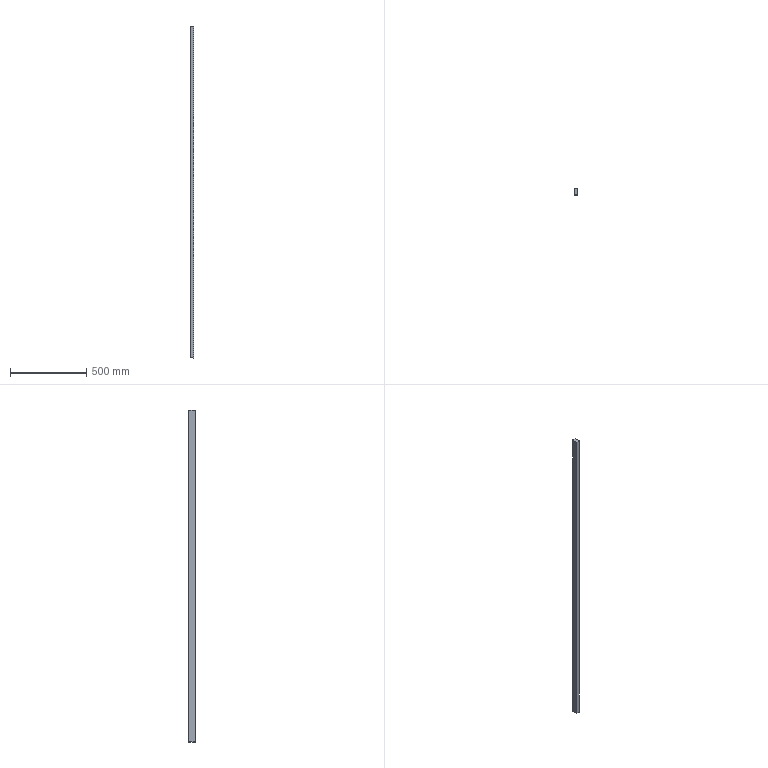Part | SolidWorks | features Extrusion 1 | 1 solid | 6 faces | box 25 x 40 x 2181 mm | volume 2180980 mm3 | plane 6
STEP:
#1=CARTESIAN_POINT('',(-110.,20.,2180.98));
#2=VERTEX_POINT('',#1);
#3=CARTESIAN_POINT('',(-110.,20.,0.));
#4=VERTEX_POINT('',#3);
#5=CARTESIAN_POINT('',(-110.,20.,2228.15));
#6=DIRECTION('',(0.,0.,-1.));
#7=VECTOR('',#6,1000.);
#8=LINE('',#5,#7);
#9=EDGE_CURVE('',#2,#4,#8,.T.);
#10=ORIENTED_EDGE('',*,*,#9,.F.);
#11=CARTESIAN_POINT('',(-85.,20.,2180.98));
#12=VERTEX_POINT('',#11);
#13=CARTESIAN_POINT('',(0.,20.,2180.98));
#14=DIRECTION('',(1.,0.,0.));
#15=VECTOR('',#14,1000.);
#16=LINE('',#13,#15);
#17=EDGE_CURVE('',#2,#12,#16,.T.);
#18=ORIENTED_EDGE('',*,*,#17,.T.);
#19=CARTESIAN_POINT('',(-85.,20.,0.));
#20=VERTEX_POINT('',#19);
#21=CARTESIAN_POINT('',(-85.,20.,2228.15));
#22=DIRECTION('',(0.,0.,-1.));
#23=VECTOR('',#22,1000.);
#24=LINE('',#21,#23);
#25=EDGE_CURVE('',#12,#20,#24,.T.);
#26=ORIENTED_EDGE('',*,*,#25,.T.);
#27=CARTESIAN_POINT('',(0.,20.,0.));
#28=DIRECTION('',(-1.,0.,0.));
#29=VECTOR('',#28,1000.);
#30=LINE('',#27,#29);
#31=EDGE_CURVE('',#20,#4,#30,.T.);
#32=ORIENTED_EDGE('',*,*,#31,.T.);
#33=EDGE_LOOP('',(#10,#18,#26,#32));
#34=FACE_OUTER_BOUND('',#33,.T.);
#35=CARTESIAN_POINT('',(0.,20.,2228.15));
#36=DIRECTION('',(0.,-1.,0.));
#37=DIRECTION('',(1.,0.,0.));
#38=AXIS2_PLACEMENT_3D('',#35,#36,#37);
#39=PLANE('',#38);
#40=ADVANCED_FACE('',(#34),#39,.F.);
#41=CARTESIAN_POINT('',(-110.,-20.,2180.98));
#42=VERTEX_POINT('',#41);
#43=CARTESIAN_POINT('',(-110.,-20.,0.));
#44=VERTEX_POINT('',#43);
#45=CARTESIAN_POINT('',(-110.,-20.,2228.15));
#46=DIRECTION('',(0.,0.,-1.));
#47=VECTOR('',#46,1000.);
#48=LINE('',#45,#47);
#49=EDGE_CURVE('',#42,#44,#48,.T.);
#50=ORIENTED_EDGE('',*,*,#49,.F.);
#51=CARTESIAN_POINT('',(-110.,0.,2180.98));
#52=DIRECTION('',(0.,1.,0.));
#53=VECTOR('',#52,1000.);
#54=LINE('',#51,#53);
#55=EDGE_CURVE('',#42,#2,#54,.T.);
#56=ORIENTED_EDGE('',*,*,#55,.T.);
#57=ORIENTED_EDGE('',*,*,#9,.T.);
#58=CARTESIAN_POINT('',(-110.,0.,0.));
#59=DIRECTION('',(0.,-1.,0.));
#60=VECTOR('',#59,1000.);
#61=LINE('',#58,#60);
#62=EDGE_CURVE('',#4,#44,#61,.T.);
#63=ORIENTED_EDGE('',*,*,#62,.T.);
#64=EDGE_LOOP('',(#50,#56,#57,#63));
#65=FACE_OUTER_BOUND('',#64,.T.);
#66=CARTESIAN_POINT('',(-110.,0.,2228.15));
#67=DIRECTION('',(1.,0.,0.));
#68=DIRECTION('',(0.,1.,0.));
#69=AXIS2_PLACEMENT_3D('',#66,#67,#68);
#70=PLANE('',#69);
#71=ADVANCED_FACE('',(#65),#70,.F.);
#72=CARTESIAN_POINT('',(-85.,-20.,2180.98));
#73=VERTEX_POINT('',#72);
#74=CARTESIAN_POINT('',(0.,-20.,2180.98));
#75=DIRECTION('',(1.,0.,0.));
#76=VECTOR('',#75,1000.);
#77=LINE('',#74,#76);
#78=EDGE_CURVE('',#42,#73,#77,.T.);
#79=ORIENTED_EDGE('',*,*,#78,.F.);
#80=ORIENTED_EDGE('',*,*,#49,.T.);
#81=CARTESIAN_POINT('',(-85.,-20.,0.));
#82=VERTEX_POINT('',#81);
#83=CARTESIAN_POINT('',(0.,-20.,0.));
#84=DIRECTION('',(-1.,0.,0.));
#85=VECTOR('',#84,1000.);
#86=LINE('',#83,#85);
#87=EDGE_CURVE('',#82,#44,#86,.T.);
#88=ORIENTED_EDGE('',*,*,#87,.F.);
#89=CARTESIAN_POINT('',(-85.,-20.,2228.15));
#90=DIRECTION('',(0.,0.,-1.));
#91=VECTOR('',#90,1000.);
#92=LINE('',#89,#91);
#93=EDGE_CURVE('',#73,#82,#92,.T.);
#94=ORIENTED_EDGE('',*,*,#93,.F.);
#95=EDGE_LOOP('',(#79,#80,#88,#94));
#96=FACE_OUTER_BOUND('',#95,.T.);
#97=CARTESIAN_POINT('',(0.,-20.,2228.15));
#98=DIRECTION('',(0.,-1.,0.));
#99=DIRECTION('',(1.,0.,0.));
#100=AXIS2_PLACEMENT_3D('',#97,#98,#99);
#101=PLANE('',#100);
#102=ADVANCED_FACE('',(#96),#101,.T.);
#103=CARTESIAN_POINT('',(-85.,0.,2180.98));
#104=DIRECTION('',(0.,1.,0.));
#105=VECTOR('',#104,1000.);
#106=LINE('',#103,#105);
#107=EDGE_CURVE('',#73,#12,#106,.T.);
#108=ORIENTED_EDGE('',*,*,#107,.F.);
#109=ORIENTED_EDGE('',*,*,#93,.T.);
#110=CARTESIAN_POINT('',(-85.,0.,0.));
#111=DIRECTION('',(0.,-1.,0.));
#112=VECTOR('',#111,1000.);
#113=LINE('',#110,#112);
#114=EDGE_CURVE('',#20,#82,#113,.T.);
#115=ORIENTED_EDGE('',*,*,#114,.F.);
#116=ORIENTED_EDGE('',*,*,#25,.F.);
#117=EDGE_LOOP('',(#108,#109,#115,#116));
#118=FACE_OUTER_BOUND('',#117,.T.);
#119=CARTESIAN_POINT('',(-85.,0.,2228.15));
#120=DIRECTION('',(1.,0.,0.));
#121=DIRECTION('',(0.,1.,0.));
#122=AXIS2_PLACEMENT_3D('',#119,#120,#121);
#123=PLANE('',#122);
#124=ADVANCED_FACE('',(#118),#123,.T.);
#125=ORIENTED_EDGE('',*,*,#31,.F.);
#126=ORIENTED_EDGE('',*,*,#114,.T.);
#127=ORIENTED_EDGE('',*,*,#87,.T.);
#128=ORIENTED_EDGE('',*,*,#62,.F.);
#129=EDGE_LOOP('',(#125,#126,#127,#128));
#130=FACE_OUTER_BOUND('',#129,.T.);
#131=CARTESIAN_POINT('',(0.,0.,0.));
#132=DIRECTION('',(0.,0.,1.));
#133=DIRECTION('',(1.,0.,0.));
#134=AXIS2_PLACEMENT_3D('',#131,#132,#133);
#135=PLANE('',#134);
#136=ADVANCED_FACE('',(#130),#135,.F.);
#137=ORIENTED_EDGE('',*,*,#55,.F.);
#138=ORIENTED_EDGE('',*,*,#78,.T.);
#139=ORIENTED_EDGE('',*,*,#107,.T.);
#140=ORIENTED_EDGE('',*,*,#17,.F.);
#141=EDGE_LOOP('',(#137,#138,#139,#140));
#142=FACE_OUTER_BOUND('',#141,.T.);
#143=CARTESIAN_POINT('',(1.672,-1.37,2180.98));
#144=DIRECTION('',(0.,0.,-1.));
#145=DIRECTION('',(-1.,0.,0.));
#146=AXIS2_PLACEMENT_3D('',#143,#144,#145);
#147=PLANE('',#146);
#148=ADVANCED_FACE('',(#142),#147,.F.);
#149=CLOSED_SHELL('',(#40,#71,#102,#124,#136,#148));
#150=MANIFOLD_SOLID_BREP('',#149);
#151=CARTESIAN_POINT('',(0.,0.,0.));
#152=DIRECTION('',(0.,0.,1.));
#153=DIRECTION('',(1.,0.,0.));
#154=AXIS2_PLACEMENT_3D('',#151,#152,#153);
#155=(LENGTH_UNIT()NAMED_UNIT(*)SI_UNIT(.MILLI.,.METRE.));
#156=UNCERTAINTY_MEASURE_WITH_UNIT(LENGTH_MEASURE(0.00001),#155,'','');
#157=(NAMED_UNIT(*)PLANE_ANGLE_UNIT()SI_UNIT($,.RADIAN.));
#158=(NAMED_UNIT(*)SI_UNIT($,.STERADIAN.)SOLID_ANGLE_UNIT());
#159=(GEOMETRIC_REPRESENTATION_CONTEXT(3)GLOBAL_UNCERTAINTY_ASSIGNED_CONTEXT((#156))GLOBAL_UNIT_ASSIGNED_CONTEXT((#155,#157,#158))REPRESENTATION_CONTEXT('',''));
#160=ADVANCED_BREP_SHAPE_REPRESENTATION('',(#150,#154),#159);